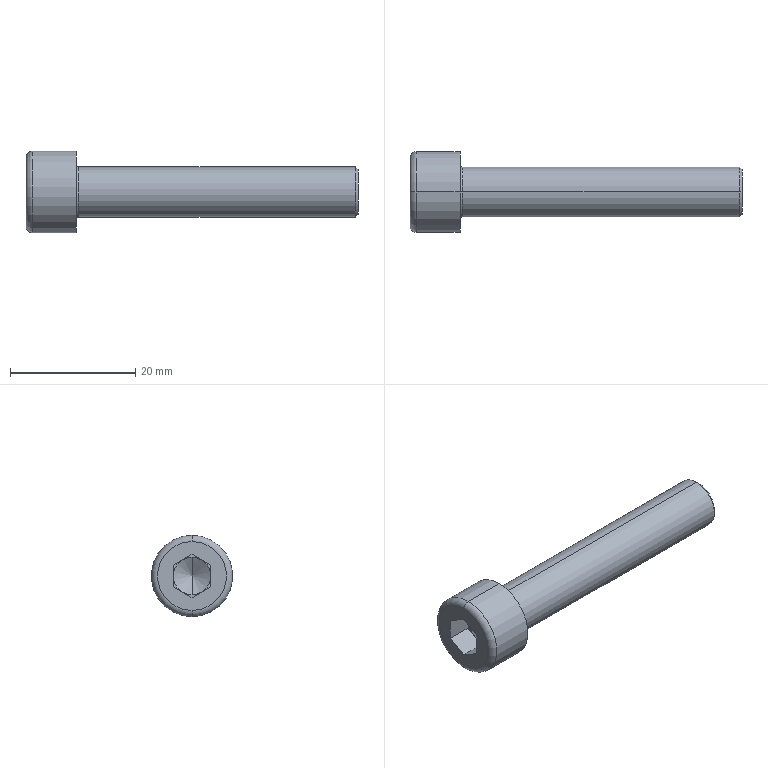Part | NX | features BREP 1 | 1 solid | 27 faces | box 53 x 13 x 13 mm | volume 3173 mm3 | plane 15 | torus 4 | cylinder 4 | cone 4 | commonest cylinder face diameters 8 x2 13 x2
STEP:
#1=CARTESIAN_POINT('',(8.4,0.,4.));
#2=VERTEX_POINT('',#1);
#3=CARTESIAN_POINT('',(8.,0.,4.4));
#4=VERTEX_POINT('',#3);
#5=CARTESIAN_POINT('',(8.4,0.,4.4));
#6=DIRECTION('',(0.,1.,0.));
#7=DIRECTION('',(0.,0.,1.));
#8=AXIS2_PLACEMENT_3D('',#5,#6,#7);
#9=CIRCLE('',#8,0.4);
#10=EDGE_CURVE('',#2,#4,#9,.T.);
#11=ORIENTED_EDGE('',*,*,#10,.F.);
#12=CARTESIAN_POINT('',(8.4,0.,-4.));
#13=VERTEX_POINT('',#12);
#14=CARTESIAN_POINT('',(8.4,0.,0.));
#15=DIRECTION('',(1.,0.,0.));
#16=DIRECTION('',(0.,0.,-1.));
#17=AXIS2_PLACEMENT_3D('',#14,#15,#16);
#18=CIRCLE('',#17,4.);
#19=EDGE_CURVE('',#13,#2,#18,.T.);
#20=ORIENTED_EDGE('',*,*,#19,.F.);
#21=CARTESIAN_POINT('',(8.,0.,-4.4));
#22=VERTEX_POINT('',#21);
#23=CARTESIAN_POINT('',(8.4,0.,-4.4));
#24=DIRECTION('',(0.,-1.,0.));
#25=DIRECTION('',(0.,0.,-1.));
#26=AXIS2_PLACEMENT_3D('',#23,#24,#25);
#27=CIRCLE('',#26,0.4);
#28=EDGE_CURVE('',#13,#22,#27,.T.);
#29=ORIENTED_EDGE('',*,*,#28,.T.);
#30=CARTESIAN_POINT('',(8.,0.,0.));
#31=DIRECTION('',(-1.,0.,0.));
#32=DIRECTION('',(0.,0.,-1.));
#33=AXIS2_PLACEMENT_3D('',#30,#31,#32);
#34=CIRCLE('',#33,4.4);
#35=EDGE_CURVE('',#4,#22,#34,.T.);
#36=ORIENTED_EDGE('',*,*,#35,.F.);
#37=EDGE_LOOP('',(#11,#20,#29,#36));
#38=FACE_BOUND('',#37,.T.);
#39=CARTESIAN_POINT('',(8.4,0.,0.));
#40=DIRECTION('',(1.,0.,0.));
#41=DIRECTION('',(0.,0.,1.));
#42=AXIS2_PLACEMENT_3D('',#39,#40,#41);
#43=TOROIDAL_SURFACE('',#42,4.4,0.4);
#44=ADVANCED_FACE('',(#38),#43,.F.);
#45=CARTESIAN_POINT('',(52.6,0.,4.));
#46=VERTEX_POINT('',#45);
#47=CARTESIAN_POINT('',(52.6,0.,-4.));
#48=VERTEX_POINT('',#47);
#49=CARTESIAN_POINT('',(52.6,0.,0.));
#50=DIRECTION('',(-1.,0.,0.));
#51=DIRECTION('',(0.,0.,-1.));
#52=AXIS2_PLACEMENT_3D('',#49,#50,#51);
#53=CIRCLE('',#52,4.);
#54=EDGE_CURVE('',#46,#48,#53,.T.);
#55=ORIENTED_EDGE('',*,*,#54,.T.);
#56=CARTESIAN_POINT('',(53.,0.,-4.));
#57=DIRECTION('',(-1.,0.,0.));
#58=VECTOR('',#57,1000.);
#59=LINE('',#56,#58);
#60=EDGE_CURVE('',#48,#13,#59,.T.);
#61=ORIENTED_EDGE('',*,*,#60,.T.);
#62=ORIENTED_EDGE('',*,*,#19,.T.);
#63=CARTESIAN_POINT('',(53.,0.,4.));
#64=DIRECTION('',(-1.,0.,0.));
#65=VECTOR('',#64,1000.);
#66=LINE('',#63,#65);
#67=EDGE_CURVE('',#46,#2,#66,.T.);
#68=ORIENTED_EDGE('',*,*,#67,.F.);
#69=EDGE_LOOP('',(#55,#61,#62,#68));
#70=FACE_BOUND('',#69,.T.);
#71=CARTESIAN_POINT('',(53.,0.,0.));
#72=DIRECTION('',(-1.,0.,0.));
#73=DIRECTION('',(0.,0.,-1.));
#74=AXIS2_PLACEMENT_3D('',#71,#72,#73);
#75=CYLINDRICAL_SURFACE('',#74,4.);
#76=ADVANCED_FACE('',(#70),#75,.T.);
#77=CARTESIAN_POINT('',(8.4,0.,0.));
#78=DIRECTION('',(1.,0.,0.));
#79=DIRECTION('',(0.,0.,-1.));
#80=AXIS2_PLACEMENT_3D('',#77,#78,#79);
#81=CIRCLE('',#80,4.);
#82=EDGE_CURVE('',#2,#13,#81,.T.);
#83=ORIENTED_EDGE('',*,*,#82,.F.);
#84=ORIENTED_EDGE('',*,*,#10,.T.);
#85=CARTESIAN_POINT('',(8.,0.,0.));
#86=DIRECTION('',(-1.,0.,0.));
#87=DIRECTION('',(0.,0.,-1.));
#88=AXIS2_PLACEMENT_3D('',#85,#86,#87);
#89=CIRCLE('',#88,4.4);
#90=EDGE_CURVE('',#22,#4,#89,.T.);
#91=ORIENTED_EDGE('',*,*,#90,.F.);
#92=ORIENTED_EDGE('',*,*,#28,.F.);
#93=EDGE_LOOP('',(#83,#84,#91,#92));
#94=FACE_BOUND('',#93,.T.);
#95=CARTESIAN_POINT('',(8.4,0.,0.));
#96=DIRECTION('',(1.,0.,0.));
#97=DIRECTION('',(0.,0.,1.));
#98=AXIS2_PLACEMENT_3D('',#95,#96,#97);
#99=TOROIDAL_SURFACE('',#98,4.4,0.4);
#100=ADVANCED_FACE('',(#94),#99,.F.);
#101=ORIENTED_EDGE('',*,*,#90,.T.);
#102=ORIENTED_EDGE('',*,*,#35,.T.);
#103=EDGE_LOOP('',(#101,#102));
#104=FACE_BOUND('',#103,.T.);
#105=CARTESIAN_POINT('',(8.,0.,6.5));
#106=VERTEX_POINT('',#105);
#107=CARTESIAN_POINT('',(8.,0.,-6.5));
#108=VERTEX_POINT('',#107);
#109=CARTESIAN_POINT('',(8.,0.,0.));
#110=DIRECTION('',(1.,0.,0.));
#111=DIRECTION('',(0.,0.,-1.));
#112=AXIS2_PLACEMENT_3D('',#109,#110,#111);
#113=CIRCLE('',#112,6.5);
#114=EDGE_CURVE('',#106,#108,#113,.T.);
#115=ORIENTED_EDGE('',*,*,#114,.T.);
#116=CARTESIAN_POINT('',(8.,0.,0.));
#117=DIRECTION('',(1.,0.,0.));
#118=DIRECTION('',(0.,0.,-1.));
#119=AXIS2_PLACEMENT_3D('',#116,#117,#118);
#120=CIRCLE('',#119,6.5);
#121=EDGE_CURVE('',#108,#106,#120,.T.);
#122=ORIENTED_EDGE('',*,*,#121,.T.);
#123=EDGE_LOOP('',(#115,#122));
#124=FACE_BOUND('',#123,.T.);
#125=CARTESIAN_POINT('',(8.,0.,0.));
#126=DIRECTION('',(1.,0.,0.));
#127=DIRECTION('',(0.,0.,1.));
#128=AXIS2_PLACEMENT_3D('',#125,#126,#127);
#129=PLANE('',#128);
#130=ADVANCED_FACE('',(#104,#124),#129,.T.);
#131=ORIENTED_EDGE('',*,*,#60,.F.);
#132=CARTESIAN_POINT('',(52.6,0.,0.));
#133=DIRECTION('',(-1.,0.,0.));
#134=DIRECTION('',(0.,0.,-1.));
#135=AXIS2_PLACEMENT_3D('',#132,#133,#134);
#136=CIRCLE('',#135,4.);
#137=EDGE_CURVE('',#48,#46,#136,.T.);
#138=ORIENTED_EDGE('',*,*,#137,.T.);
#139=ORIENTED_EDGE('',*,*,#67,.T.);
#140=ORIENTED_EDGE('',*,*,#82,.T.);
#141=EDGE_LOOP('',(#131,#138,#139,#140));
#142=FACE_BOUND('',#141,.T.);
#143=CARTESIAN_POINT('',(53.,0.,0.));
#144=DIRECTION('',(-1.,0.,0.));
#145=DIRECTION('',(0.,0.,-1.));
#146=AXIS2_PLACEMENT_3D('',#143,#144,#145);
#147=CYLINDRICAL_SURFACE('',#146,4.);
#148=ADVANCED_FACE('',(#142),#147,.T.);
#149=CARTESIAN_POINT('',(53.,0.,-3.6));
#150=VERTEX_POINT('',#149);
#151=CARTESIAN_POINT('',(53.,0.,3.6));
#152=VERTEX_POINT('',#151);
#153=CARTESIAN_POINT('',(53.,0.,0.));
#154=DIRECTION('',(1.,0.,0.));
#155=DIRECTION('',(0.,0.,-1.));
#156=AXIS2_PLACEMENT_3D('',#153,#154,#155);
#157=CIRCLE('',#156,3.6);
#158=EDGE_CURVE('',#150,#152,#157,.T.);
#159=ORIENTED_EDGE('',*,*,#158,.F.);
#160=CARTESIAN_POINT('',(53.,0.,-3.6));
#161=DIRECTION('',(-0.7071,0.,-0.7071));
#162=VECTOR('',#161,1000.);
#163=LINE('',#160,#162);
#164=EDGE_CURVE('',#150,#48,#163,.T.);
#165=ORIENTED_EDGE('',*,*,#164,.T.);
#166=ORIENTED_EDGE('',*,*,#54,.F.);
#167=CARTESIAN_POINT('',(53.,0.,3.6));
#168=DIRECTION('',(-0.7071,0.,0.7071));
#169=VECTOR('',#168,1000.);
#170=LINE('',#167,#169);
#171=EDGE_CURVE('',#152,#46,#170,.T.);
#172=ORIENTED_EDGE('',*,*,#171,.F.);
#173=EDGE_LOOP('',(#159,#165,#166,#172));
#174=FACE_BOUND('',#173,.T.);
#175=CARTESIAN_POINT('',(53.,0.,0.));
#176=DIRECTION('',(-1.,0.,0.));
#177=DIRECTION('',(0.,0.,-1.));
#178=AXIS2_PLACEMENT_3D('',#175,#176,#177);
#179=CONICAL_SURFACE('',#178,3.6,0.7854);
#180=ADVANCED_FACE('',(#174),#179,.T.);
#181=CARTESIAN_POINT('',(1.,0.,-6.5));
#182=VERTEX_POINT('',#181);
#183=CARTESIAN_POINT('',(8.,0.,-6.5));
#184=DIRECTION('',(-1.,0.,0.));
#185=VECTOR('',#184,1000.);
#186=LINE('',#183,#185);
#187=EDGE_CURVE('',#182,#108,#186,.F.);
#188=ORIENTED_EDGE('',*,*,#187,.T.);
#189=ORIENTED_EDGE('',*,*,#114,.F.);
#190=CARTESIAN_POINT('',(1.,0.,6.5));
#191=VERTEX_POINT('',#190);
#192=CARTESIAN_POINT('',(8.,0.,6.5));
#193=DIRECTION('',(-1.,0.,0.));
#194=VECTOR('',#193,1000.);
#195=LINE('',#192,#194);
#196=EDGE_CURVE('',#191,#106,#195,.F.);
#197=ORIENTED_EDGE('',*,*,#196,.F.);
#198=CARTESIAN_POINT('',(1.,0.,0.));
#199=DIRECTION('',(1.,0.,0.));
#200=DIRECTION('',(0.,0.,-1.));
#201=AXIS2_PLACEMENT_3D('',#198,#199,#200);
#202=CIRCLE('',#201,6.5);
#203=EDGE_CURVE('',#191,#182,#202,.T.);
#204=ORIENTED_EDGE('',*,*,#203,.T.);
#205=EDGE_LOOP('',(#188,#189,#197,#204));
#206=FACE_BOUND('',#205,.T.);
#207=CARTESIAN_POINT('',(8.,0.,0.));
#208=DIRECTION('',(-1.,0.,0.));
#209=DIRECTION('',(0.,0.,-1.));
#210=AXIS2_PLACEMENT_3D('',#207,#208,#209);
#211=CYLINDRICAL_SURFACE('',#210,6.5);
#212=ADVANCED_FACE('',(#206),#211,.T.);
#213=ORIENTED_EDGE('',*,*,#121,.F.);
#214=ORIENTED_EDGE('',*,*,#187,.F.);
#215=CARTESIAN_POINT('',(1.,0.,0.));
#216=DIRECTION('',(1.,0.,0.));
#217=DIRECTION('',(0.,0.,-1.));
#218=AXIS2_PLACEMENT_3D('',#215,#216,#217);
#219=CIRCLE('',#218,6.5);
#220=EDGE_CURVE('',#182,#191,#219,.T.);
#221=ORIENTED_EDGE('',*,*,#220,.T.);
#222=ORIENTED_EDGE('',*,*,#196,.T.);
#223=EDGE_LOOP('',(#213,#214,#221,#222));
#224=FACE_BOUND('',#223,.T.);
#225=CARTESIAN_POINT('',(8.,0.,0.));
#226=DIRECTION('',(-1.,0.,0.));
#227=DIRECTION('',(0.,0.,-1.));
#228=AXIS2_PLACEMENT_3D('',#225,#226,#227);
#229=CYLINDRICAL_SURFACE('',#228,6.5);
#230=ADVANCED_FACE('',(#224),#229,.T.);
#231=ORIENTED_EDGE('',*,*,#164,.F.);
#232=CARTESIAN_POINT('',(53.,0.,0.));
#233=DIRECTION('',(1.,0.,0.));
#234=DIRECTION('',(0.,0.,-1.));
#235=AXIS2_PLACEMENT_3D('',#232,#233,#234);
#236=CIRCLE('',#235,3.6);
#237=EDGE_CURVE('',#152,#150,#236,.T.);
#238=ORIENTED_EDGE('',*,*,#237,.F.);
#239=ORIENTED_EDGE('',*,*,#171,.T.);
#240=ORIENTED_EDGE('',*,*,#137,.F.);
#241=EDGE_LOOP('',(#231,#238,#239,#240));
#242=FACE_BOUND('',#241,.T.);
#243=CARTESIAN_POINT('',(53.,0.,0.));
#244=DIRECTION('',(-1.,0.,0.));
#245=DIRECTION('',(0.,0.,-1.));
#246=AXIS2_PLACEMENT_3D('',#243,#244,#245);
#247=CONICAL_SURFACE('',#246,3.6,0.7854);
#248=ADVANCED_FACE('',(#242),#247,.T.);
#249=ORIENTED_EDGE('',*,*,#237,.T.);
#250=ORIENTED_EDGE('',*,*,#158,.T.);
#251=EDGE_LOOP('',(#249,#250));
#252=FACE_BOUND('',#251,.T.);
#253=CARTESIAN_POINT('',(53.,0.,0.));
#254=DIRECTION('',(1.,0.,0.));
#255=DIRECTION('',(0.,0.,1.));
#256=AXIS2_PLACEMENT_3D('',#253,#254,#255);
#257=PLANE('',#256);
#258=ADVANCED_FACE('',(#252),#257,.T.);
#259=CARTESIAN_POINT('',(0.,0.,5.5));
#260=VERTEX_POINT('',#259);
#261=CARTESIAN_POINT('',(1.,0.,5.5));
#262=DIRECTION('',(0.,1.,0.));
#263=DIRECTION('',(0.,0.,1.));
#264=AXIS2_PLACEMENT_3D('',#261,#262,#263);
#265=CIRCLE('',#264,1.);
#266=EDGE_CURVE('',#260,#191,#265,.T.);
#267=ORIENTED_EDGE('',*,*,#266,.F.);
#268=CARTESIAN_POINT('',(0.,0.,-5.5));
#269=VERTEX_POINT('',#268);
#270=CARTESIAN_POINT('',(0.,0.,0.));
#271=DIRECTION('',(-1.,0.,0.));
#272=DIRECTION('',(0.,0.,-1.));
#273=AXIS2_PLACEMENT_3D('',#270,#271,#272);
#274=CIRCLE('',#273,5.5);
#275=EDGE_CURVE('',#269,#260,#274,.T.);
#276=ORIENTED_EDGE('',*,*,#275,.F.);
#277=CARTESIAN_POINT('',(1.,0.,-5.5));
#278=DIRECTION('',(0.,-1.,0.));
#279=DIRECTION('',(0.,0.,-1.));
#280=AXIS2_PLACEMENT_3D('',#277,#278,#279);
#281=CIRCLE('',#280,1.);
#282=EDGE_CURVE('',#269,#182,#281,.T.);
#283=ORIENTED_EDGE('',*,*,#282,.T.);
#284=ORIENTED_EDGE('',*,*,#203,.F.);
#285=EDGE_LOOP('',(#267,#276,#283,#284));
#286=FACE_BOUND('',#285,.T.);
#287=CARTESIAN_POINT('',(1.,0.,0.));
#288=DIRECTION('',(1.,0.,0.));
#289=DIRECTION('',(0.,0.,1.));
#290=AXIS2_PLACEMENT_3D('',#287,#288,#289);
#291=TOROIDAL_SURFACE('',#290,5.5,1.);
#292=ADVANCED_FACE('',(#286),#291,.T.);
#293=CARTESIAN_POINT('',(0.,0.,0.));
#294=DIRECTION('',(-1.,0.,0.));
#295=DIRECTION('',(0.,0.,-1.));
#296=AXIS2_PLACEMENT_3D('',#293,#294,#295);
#297=CIRCLE('',#296,5.5);
#298=EDGE_CURVE('',#260,#269,#297,.T.);
#299=ORIENTED_EDGE('',*,*,#298,.F.);
#300=ORIENTED_EDGE('',*,*,#266,.T.);
#301=ORIENTED_EDGE('',*,*,#220,.F.);
#302=ORIENTED_EDGE('',*,*,#282,.F.);
#303=EDGE_LOOP('',(#299,#300,#301,#302));
#304=FACE_BOUND('',#303,.T.);
#305=CARTESIAN_POINT('',(1.,0.,0.));
#306=DIRECTION('',(1.,0.,0.));
#307=DIRECTION('',(0.,0.,1.));
#308=AXIS2_PLACEMENT_3D('',#305,#306,#307);
#309=TOROIDAL_SURFACE('',#308,5.5,1.);
#310=ADVANCED_FACE('',(#304),#309,.T.);
#311=ORIENTED_EDGE('',*,*,#275,.T.);
#312=ORIENTED_EDGE('',*,*,#298,.T.);
#313=EDGE_LOOP('',(#311,#312));
#314=FACE_BOUND('',#313,.T.);
#315=CARTESIAN_POINT('',(0.,-3.,-1.732));
#316=VERTEX_POINT('',#315);
#317=CARTESIAN_POINT('',(0.,0.,-3.464));
#318=VERTEX_POINT('',#317);
#319=CARTESIAN_POINT('',(0.,-3.,-1.732));
#320=DIRECTION('',(0.,0.866,-0.5));
#321=VECTOR('',#320,1000.);
#322=LINE('',#319,#321);
#323=EDGE_CURVE('',#316,#318,#322,.T.);
#324=ORIENTED_EDGE('',*,*,#323,.T.);
#325=CARTESIAN_POINT('',(0.,3.,-1.732));
#326=VERTEX_POINT('',#325);
#327=CARTESIAN_POINT('',(0.,0.,-3.464));
#328=DIRECTION('',(0.,0.866,0.5));
#329=VECTOR('',#328,1000.);
#330=LINE('',#327,#329);
#331=EDGE_CURVE('',#318,#326,#330,.T.);
#332=ORIENTED_EDGE('',*,*,#331,.T.);
#333=CARTESIAN_POINT('',(0.,3.,1.732));
#334=VERTEX_POINT('',#333);
#335=CARTESIAN_POINT('',(0.,3.,-1.732));
#336=DIRECTION('',(0.,0.,1.));
#337=VECTOR('',#336,1000.);
#338=LINE('',#335,#337);
#339=EDGE_CURVE('',#326,#334,#338,.T.);
#340=ORIENTED_EDGE('',*,*,#339,.T.);
#341=CARTESIAN_POINT('',(0.,0.,3.464));
#342=VERTEX_POINT('',#341);
#343=CARTESIAN_POINT('',(0.,3.,1.732));
#344=DIRECTION('',(0.,-0.866,0.5));
#345=VECTOR('',#344,1000.);
#346=LINE('',#343,#345);
#347=EDGE_CURVE('',#334,#342,#346,.T.);
#348=ORIENTED_EDGE('',*,*,#347,.T.);
#349=CARTESIAN_POINT('',(0.,-3.,1.732));
#350=VERTEX_POINT('',#349);
#351=CARTESIAN_POINT('',(0.,0.,3.464));
#352=DIRECTION('',(0.,-0.866,-0.5));
#353=VECTOR('',#352,1000.);
#354=LINE('',#351,#353);
#355=EDGE_CURVE('',#342,#350,#354,.T.);
#356=ORIENTED_EDGE('',*,*,#355,.T.);
#357=CARTESIAN_POINT('',(0.,-3.,1.732));
#358=DIRECTION('',(0.,0.,-1.));
#359=VECTOR('',#358,1000.);
#360=LINE('',#357,#359);
#361=EDGE_CURVE('',#350,#316,#360,.T.);
#362=ORIENTED_EDGE('',*,*,#361,.T.);
#363=EDGE_LOOP('',(#324,#332,#340,#348,#356,#362));
#364=FACE_BOUND('',#363,.T.);
#365=CARTESIAN_POINT('',(0.,0.,0.));
#366=DIRECTION('',(1.,0.,0.));
#367=DIRECTION('',(0.,0.,1.));
#368=AXIS2_PLACEMENT_3D('',#365,#366,#367);
#369=PLANE('',#368);
#370=ADVANCED_FACE('',(#314,#364),#369,.F.);
#371=ORIENTED_EDGE('',*,*,#361,.F.);
#372=CARTESIAN_POINT('',(4.,-3.,1.732));
#373=VERTEX_POINT('',#372);
#374=CARTESIAN_POINT('',(4.,-3.,1.732));
#375=DIRECTION('',(-1.,0.,0.));
#376=VECTOR('',#375,1000.);
#377=LINE('',#374,#376);
#378=EDGE_CURVE('',#373,#350,#377,.T.);
#379=ORIENTED_EDGE('',*,*,#378,.F.);
#380=CARTESIAN_POINT('',(4.,-3.,0.));
#381=VERTEX_POINT('',#380);
#382=CARTESIAN_POINT('',(4.,-3.,1.732));
#383=DIRECTION('',(0.,0.,-1.));
#384=VECTOR('',#383,1000.);
#385=LINE('',#382,#384);
#386=EDGE_CURVE('',#373,#381,#385,.T.);
#387=ORIENTED_EDGE('',*,*,#386,.T.);
#388=CARTESIAN_POINT('',(4.,-3.,-1.732));
#389=VERTEX_POINT('',#388);
#390=CARTESIAN_POINT('',(4.,-3.,1.732));
#391=DIRECTION('',(0.,0.,-1.));
#392=VECTOR('',#391,1000.);
#393=LINE('',#390,#392);
#394=EDGE_CURVE('',#381,#389,#393,.T.);
#395=ORIENTED_EDGE('',*,*,#394,.T.);
#396=CARTESIAN_POINT('',(4.,-3.,-1.732));
#397=DIRECTION('',(-1.,0.,0.));
#398=VECTOR('',#397,1000.);
#399=LINE('',#396,#398);
#400=EDGE_CURVE('',#389,#316,#399,.T.);
#401=ORIENTED_EDGE('',*,*,#400,.T.);
#402=EDGE_LOOP('',(#371,#379,#387,#395,#401));
#403=FACE_BOUND('',#402,.T.);
#404=CARTESIAN_POINT('',(4.,-3.,1.732));
#405=DIRECTION('',(0.,1.,0.));
#406=DIRECTION('',(0.,0.,-1.));
#407=AXIS2_PLACEMENT_3D('',#404,#405,#406);
#408=PLANE('',#407);
#409=ADVANCED_FACE('',(#403),#408,.T.);
#410=ORIENTED_EDGE('',*,*,#347,.F.);
#411=CARTESIAN_POINT('',(4.,3.,1.732));
#412=VERTEX_POINT('',#411);
#413=CARTESIAN_POINT('',(4.,3.,1.732));
#414=DIRECTION('',(-1.,0.,0.));
#415=VECTOR('',#414,1000.);
#416=LINE('',#413,#415);
#417=EDGE_CURVE('',#412,#334,#416,.T.);
#418=ORIENTED_EDGE('',*,*,#417,.F.);
#419=CARTESIAN_POINT('',(4.,1.5,2.598));
#420=VERTEX_POINT('',#419);
#421=CARTESIAN_POINT('',(4.,3.,1.732));
#422=DIRECTION('',(0.,-0.866,0.5));
#423=VECTOR('',#422,1000.);
#424=LINE('',#421,#423);
#425=EDGE_CURVE('',#412,#420,#424,.T.);
#426=ORIENTED_EDGE('',*,*,#425,.T.);
#427=CARTESIAN_POINT('',(4.,0.,3.464));
#428=VERTEX_POINT('',#427);
#429=CARTESIAN_POINT('',(4.,3.,1.732));
#430=DIRECTION('',(0.,-0.866,0.5));
#431=VECTOR('',#430,1000.);
#432=LINE('',#429,#431);
#433=EDGE_CURVE('',#420,#428,#432,.T.);
#434=ORIENTED_EDGE('',*,*,#433,.T.);
#435=CARTESIAN_POINT('',(4.,0.,3.464));
#436=DIRECTION('',(-1.,0.,0.));
#437=VECTOR('',#436,1000.);
#438=LINE('',#435,#437);
#439=EDGE_CURVE('',#428,#342,#438,.T.);
#440=ORIENTED_EDGE('',*,*,#439,.T.);
#441=EDGE_LOOP('',(#410,#418,#426,#434,#440));
#442=FACE_BOUND('',#441,.T.);
#443=CARTESIAN_POINT('',(4.,3.,1.732));
#444=DIRECTION('',(0.,-0.5,-0.866));
#445=DIRECTION('',(0.,-0.866,0.5));
#446=AXIS2_PLACEMENT_3D('',#443,#444,#445);
#447=PLANE('',#446);
#448=ADVANCED_FACE('',(#442),#447,.T.);
#449=ORIENTED_EDGE('',*,*,#331,.F.);
#450=CARTESIAN_POINT('',(4.,0.,-3.464));
#451=VERTEX_POINT('',#450);
#452=CARTESIAN_POINT('',(4.,0.,-3.464));
#453=DIRECTION('',(-1.,0.,0.));
#454=VECTOR('',#453,1000.);
#455=LINE('',#452,#454);
#456=EDGE_CURVE('',#451,#318,#455,.T.);
#457=ORIENTED_EDGE('',*,*,#456,.F.);
#458=CARTESIAN_POINT('',(4.,1.5,-2.598));
#459=VERTEX_POINT('',#458);
#460=CARTESIAN_POINT('',(4.,0.,-3.464));
#461=DIRECTION('',(0.,0.866,0.5));
#462=VECTOR('',#461,1000.);
#463=LINE('',#460,#462);
#464=EDGE_CURVE('',#451,#459,#463,.T.);
#465=ORIENTED_EDGE('',*,*,#464,.T.);
#466=CARTESIAN_POINT('',(4.,3.,-1.732));
#467=VERTEX_POINT('',#466);
#468=CARTESIAN_POINT('',(4.,0.,-3.464));
#469=DIRECTION('',(0.,0.866,0.5));
#470=VECTOR('',#469,1000.);
#471=LINE('',#468,#470);
#472=EDGE_CURVE('',#459,#467,#471,.T.);
#473=ORIENTED_EDGE('',*,*,#472,.T.);
#474=CARTESIAN_POINT('',(4.,3.,-1.732));
#475=DIRECTION('',(-1.,0.,0.));
#476=VECTOR('',#475,1000.);
#477=LINE('',#474,#476);
#478=EDGE_CURVE('',#467,#326,#477,.T.);
#479=ORIENTED_EDGE('',*,*,#478,.T.);
#480=EDGE_LOOP('',(#449,#457,#465,#473,#479));
#481=FACE_BOUND('',#480,.T.);
#482=CARTESIAN_POINT('',(4.,0.,-3.464));
#483=DIRECTION('',(0.,-0.5,0.866));
#484=DIRECTION('',(0.,0.866,0.5));
#485=AXIS2_PLACEMENT_3D('',#482,#483,#484);
#486=PLANE('',#485);
#487=ADVANCED_FACE('',(#481),#486,.T.);
#488=ORIENTED_EDGE('',*,*,#323,.F.);
#489=ORIENTED_EDGE('',*,*,#400,.F.);
#490=CARTESIAN_POINT('',(4.,-1.5,-2.598));
#491=VERTEX_POINT('',#490);
#492=CARTESIAN_POINT('',(4.,-3.,-1.732));
#493=DIRECTION('',(0.,0.866,-0.5));
#494=VECTOR('',#493,1000.);
#495=LINE('',#492,#494);
#496=EDGE_CURVE('',#389,#491,#495,.T.);
#497=ORIENTED_EDGE('',*,*,#496,.T.);
#498=CARTESIAN_POINT('',(4.,-3.,-1.732));
#499=DIRECTION('',(0.,0.866,-0.5));
#500=VECTOR('',#499,1000.);
#501=LINE('',#498,#500);
#502=EDGE_CURVE('',#491,#451,#501,.T.);
#503=ORIENTED_EDGE('',*,*,#502,.T.);
#504=ORIENTED_EDGE('',*,*,#456,.T.);
#505=EDGE_LOOP('',(#488,#489,#497,#503,#504));
#506=FACE_BOUND('',#505,.T.);
#507=CARTESIAN_POINT('',(4.,-3.,-1.732));
#508=DIRECTION('',(0.,0.5,0.866));
#509=DIRECTION('',(0.,0.866,-0.5));
#510=AXIS2_PLACEMENT_3D('',#507,#508,#509);
#511=PLANE('',#510);
#512=ADVANCED_FACE('',(#506),#511,.T.);
#513=ORIENTED_EDGE('',*,*,#339,.F.);
#514=ORIENTED_EDGE('',*,*,#478,.F.);
#515=CARTESIAN_POINT('',(4.,3.,0.));
#516=VERTEX_POINT('',#515);
#517=CARTESIAN_POINT('',(4.,3.,-1.732));
#518=DIRECTION('',(0.,0.,1.));
#519=VECTOR('',#518,1000.);
#520=LINE('',#517,#519);
#521=EDGE_CURVE('',#467,#516,#520,.T.);
#522=ORIENTED_EDGE('',*,*,#521,.T.);
#523=CARTESIAN_POINT('',(4.,3.,-1.732));
#524=DIRECTION('',(0.,0.,1.));
#525=VECTOR('',#524,1000.);
#526=LINE('',#523,#525);
#527=EDGE_CURVE('',#516,#412,#526,.T.);
#528=ORIENTED_EDGE('',*,*,#527,.T.);
#529=ORIENTED_EDGE('',*,*,#417,.T.);
#530=EDGE_LOOP('',(#513,#514,#522,#528,#529));
#531=FACE_BOUND('',#530,.T.);
#532=CARTESIAN_POINT('',(4.,3.,-1.732));
#533=DIRECTION('',(0.,-1.,0.));
#534=DIRECTION('',(0.,0.,1.));
#535=AXIS2_PLACEMENT_3D('',#532,#533,#534);
#536=PLANE('',#535);
#537=ADVANCED_FACE('',(#531),#536,.T.);
#538=ORIENTED_EDGE('',*,*,#355,.F.);
#539=ORIENTED_EDGE('',*,*,#439,.F.);
#540=CARTESIAN_POINT('',(4.,-1.5,2.598));
#541=VERTEX_POINT('',#540);
#542=CARTESIAN_POINT('',(4.,0.,3.464));
#543=DIRECTION('',(0.,-0.866,-0.5));
#544=VECTOR('',#543,1000.);
#545=LINE('',#542,#544);
#546=EDGE_CURVE('',#428,#541,#545,.T.);
#547=ORIENTED_EDGE('',*,*,#546,.T.);
#548=CARTESIAN_POINT('',(4.,0.,3.464));
#549=DIRECTION('',(0.,-0.866,-0.5));
#550=VECTOR('',#549,1000.);
#551=LINE('',#548,#550);
#552=EDGE_CURVE('',#541,#373,#551,.T.);
#553=ORIENTED_EDGE('',*,*,#552,.T.);
#554=ORIENTED_EDGE('',*,*,#378,.T.);
#555=EDGE_LOOP('',(#538,#539,#547,#553,#554));
#556=FACE_BOUND('',#555,.T.);
#557=CARTESIAN_POINT('',(4.,0.,3.464));
#558=DIRECTION('',(0.,0.5,-0.866));
#559=DIRECTION('',(0.,-0.866,-0.5));
#560=AXIS2_PLACEMENT_3D('',#557,#558,#559);
#561=PLANE('',#560);
#562=ADVANCED_FACE('',(#556),#561,.T.);
#563=ORIENTED_EDGE('',*,*,#552,.F.);
#564=CARTESIAN_POINT('',(4.,0.,0.));
#565=DIRECTION('',(1.,0.,0.));
#566=DIRECTION('',(0.,0.,-1.));
#567=AXIS2_PLACEMENT_3D('',#564,#565,#566);
#568=CIRCLE('',#567,3.);
#569=EDGE_CURVE('',#541,#381,#568,.T.);
#570=ORIENTED_EDGE('',*,*,#569,.T.);
#571=ORIENTED_EDGE('',*,*,#386,.F.);
#572=EDGE_LOOP('',(#563,#570,#571));
#573=FACE_BOUND('',#572,.T.);
#574=CARTESIAN_POINT('',(4.,0.,-3.464));
#575=DIRECTION('',(1.,0.,0.));
#576=DIRECTION('',(0.,0.,1.));
#577=AXIS2_PLACEMENT_3D('',#574,#575,#576);
#578=PLANE('',#577);
#579=ADVANCED_FACE('',(#573),#578,.F.);
#580=ORIENTED_EDGE('',*,*,#394,.F.);
#581=CARTESIAN_POINT('',(4.,0.,0.));
#582=DIRECTION('',(1.,0.,0.));
#583=DIRECTION('',(0.,0.,-1.));
#584=AXIS2_PLACEMENT_3D('',#581,#582,#583);
#585=CIRCLE('',#584,3.);
#586=EDGE_CURVE('',#381,#491,#585,.T.);
#587=ORIENTED_EDGE('',*,*,#586,.T.);
#588=ORIENTED_EDGE('',*,*,#496,.F.);
#589=EDGE_LOOP('',(#580,#587,#588));
#590=FACE_BOUND('',#589,.T.);
#591=CARTESIAN_POINT('',(4.,0.,-3.464));
#592=DIRECTION('',(1.,0.,0.));
#593=DIRECTION('',(0.,0.,1.));
#594=AXIS2_PLACEMENT_3D('',#591,#592,#593);
#595=PLANE('',#594);
#596=ADVANCED_FACE('',(#590),#595,.F.);
#597=ORIENTED_EDGE('',*,*,#527,.F.);
#598=CARTESIAN_POINT('',(4.,0.,0.));
#599=DIRECTION('',(1.,0.,0.));
#600=DIRECTION('',(0.,0.,-1.));
#601=AXIS2_PLACEMENT_3D('',#598,#599,#600);
#602=CIRCLE('',#601,3.);
#603=EDGE_CURVE('',#516,#420,#602,.T.);
#604=ORIENTED_EDGE('',*,*,#603,.T.);
#605=ORIENTED_EDGE('',*,*,#425,.F.);
#606=EDGE_LOOP('',(#597,#604,#605));
#607=FACE_BOUND('',#606,.T.);
#608=CARTESIAN_POINT('',(4.,0.,-3.464));
#609=DIRECTION('',(1.,0.,0.));
#610=DIRECTION('',(0.,0.,1.));
#611=AXIS2_PLACEMENT_3D('',#608,#609,#610);
#612=PLANE('',#611);
#613=ADVANCED_FACE('',(#607),#612,.F.);
#614=ORIENTED_EDGE('',*,*,#433,.F.);
#615=CARTESIAN_POINT('',(4.,0.,3.));
#616=VERTEX_POINT('',#615);
#617=CARTESIAN_POINT('',(4.,0.,0.));
#618=DIRECTION('',(1.,0.,0.));
#619=DIRECTION('',(0.,0.,-1.));
#620=AXIS2_PLACEMENT_3D('',#617,#618,#619);
#621=CIRCLE('',#620,3.);
#622=EDGE_CURVE('',#420,#616,#621,.T.);
#623=ORIENTED_EDGE('',*,*,#622,.T.);
#624=CARTESIAN_POINT('',(4.,0.,0.));
#625=DIRECTION('',(1.,0.,0.));
#626=DIRECTION('',(0.,0.,-1.));
#627=AXIS2_PLACEMENT_3D('',#624,#625,#626);
#628=CIRCLE('',#627,3.);
#629=EDGE_CURVE('',#616,#541,#628,.T.);
#630=ORIENTED_EDGE('',*,*,#629,.T.);
#631=ORIENTED_EDGE('',*,*,#546,.F.);
#632=EDGE_LOOP('',(#614,#623,#630,#631));
#633=FACE_BOUND('',#632,.T.);
#634=CARTESIAN_POINT('',(4.,0.,-3.464));
#635=DIRECTION('',(1.,0.,0.));
#636=DIRECTION('',(0.,0.,1.));
#637=AXIS2_PLACEMENT_3D('',#634,#635,#636);
#638=PLANE('',#637);
#639=ADVANCED_FACE('',(#633),#638,.F.);
#640=ORIENTED_EDGE('',*,*,#472,.F.);
#641=CARTESIAN_POINT('',(4.,0.,0.));
#642=DIRECTION('',(1.,0.,0.));
#643=DIRECTION('',(0.,0.,-1.));
#644=AXIS2_PLACEMENT_3D('',#641,#642,#643);
#645=CIRCLE('',#644,3.);
#646=EDGE_CURVE('',#459,#516,#645,.T.);
#647=ORIENTED_EDGE('',*,*,#646,.T.);
#648=ORIENTED_EDGE('',*,*,#521,.F.);
#649=EDGE_LOOP('',(#640,#647,#648));
#650=FACE_BOUND('',#649,.T.);
#651=CARTESIAN_POINT('',(4.,0.,-3.464));
#652=DIRECTION('',(1.,0.,0.));
#653=DIRECTION('',(0.,0.,1.));
#654=AXIS2_PLACEMENT_3D('',#651,#652,#653);
#655=PLANE('',#654);
#656=ADVANCED_FACE('',(#650),#655,.F.);
#657=ORIENTED_EDGE('',*,*,#502,.F.);
#658=CARTESIAN_POINT('',(4.,0.,-3.));
#659=VERTEX_POINT('',#658);
#660=CARTESIAN_POINT('',(4.,0.,0.));
#661=DIRECTION('',(1.,0.,0.));
#662=DIRECTION('',(0.,0.,-1.));
#663=AXIS2_PLACEMENT_3D('',#660,#661,#662);
#664=CIRCLE('',#663,3.);
#665=EDGE_CURVE('',#491,#659,#664,.T.);
#666=ORIENTED_EDGE('',*,*,#665,.T.);
#667=CARTESIAN_POINT('',(4.,0.,0.));
#668=DIRECTION('',(1.,0.,0.));
#669=DIRECTION('',(0.,0.,-1.));
#670=AXIS2_PLACEMENT_3D('',#667,#668,#669);
#671=CIRCLE('',#670,3.);
#672=EDGE_CURVE('',#659,#459,#671,.T.);
#673=ORIENTED_EDGE('',*,*,#672,.T.);
#674=ORIENTED_EDGE('',*,*,#464,.F.);
#675=EDGE_LOOP('',(#657,#666,#673,#674));
#676=FACE_BOUND('',#675,.T.);
#677=CARTESIAN_POINT('',(4.,0.,-3.464));
#678=DIRECTION('',(1.,0.,0.));
#679=DIRECTION('',(0.,0.,1.));
#680=AXIS2_PLACEMENT_3D('',#677,#678,#679);
#681=PLANE('',#680);
#682=ADVANCED_FACE('',(#676),#681,.F.);
#683=CARTESIAN_POINT('',(5.732,0.,0.));
#684=VERTEX_POINT('',#683);
#685=CARTESIAN_POINT('',(4.,0.,3.));
#686=DIRECTION('',(-0.5,0.,0.866));
#687=VECTOR('',#686,1000.);
#688=LINE('',#685,#687);
#689=EDGE_CURVE('',#684,#616,#688,.T.);
#690=ORIENTED_EDGE('',*,*,#689,.F.);
#691=CARTESIAN_POINT('',(4.,0.,-3.));
#692=DIRECTION('',(-0.5,0.,-0.866));
#693=VECTOR('',#692,1000.);
#694=LINE('',#691,#693);
#695=EDGE_CURVE('',#684,#659,#694,.T.);
#696=ORIENTED_EDGE('',*,*,#695,.T.);
#697=ORIENTED_EDGE('',*,*,#665,.F.);
#698=ORIENTED_EDGE('',*,*,#586,.F.);
#699=ORIENTED_EDGE('',*,*,#569,.F.);
#700=ORIENTED_EDGE('',*,*,#629,.F.);
#701=EDGE_LOOP('',(#690,#696,#697,#698,#699,#700));
#702=FACE_BOUND('',#701,.T.);
#703=CARTESIAN_POINT('',(4.,0.,0.));
#704=DIRECTION('',(-1.,0.,0.));
#705=DIRECTION('',(0.,0.,-1.));
#706=AXIS2_PLACEMENT_3D('',#703,#704,#705);
#707=CONICAL_SURFACE('',#706,3.,1.047);
#708=ADVANCED_FACE('',(#702),#707,.F.);
#709=ORIENTED_EDGE('',*,*,#695,.F.);
#710=ORIENTED_EDGE('',*,*,#689,.T.);
#711=ORIENTED_EDGE('',*,*,#622,.F.);
#712=ORIENTED_EDGE('',*,*,#603,.F.);
#713=ORIENTED_EDGE('',*,*,#646,.F.);
#714=ORIENTED_EDGE('',*,*,#672,.F.);
#715=EDGE_LOOP('',(#709,#710,#711,#712,#713,#714));
#716=FACE_BOUND('',#715,.T.);
#717=CARTESIAN_POINT('',(4.,0.,0.));
#718=DIRECTION('',(-1.,0.,0.));
#719=DIRECTION('',(0.,0.,-1.));
#720=AXIS2_PLACEMENT_3D('',#717,#718,#719);
#721=CONICAL_SURFACE('',#720,3.,1.047);
#722=ADVANCED_FACE('',(#716),#721,.F.);
#723=CLOSED_SHELL('',(#44,#76,#100,#130,#148,#180,#212,#230,#248,#258,#292,#310,#370,#409,#448,#487,#512,#537,#562,#579,#596,#613,#639,#656,#682,#708,#722));
#724=MANIFOLD_SOLID_BREP('',#723);
#725=(LENGTH_UNIT()NAMED_UNIT(*)SI_UNIT(.MILLI.,.METRE.));
#726=UNCERTAINTY_MEASURE_WITH_UNIT(LENGTH_MEASURE(0.00001),#725,'','');
#727=(NAMED_UNIT(*)PLANE_ANGLE_UNIT()SI_UNIT($,.RADIAN.));
#728=(NAMED_UNIT(*)SI_UNIT($,.STERADIAN.)SOLID_ANGLE_UNIT());
#729=(GEOMETRIC_REPRESENTATION_CONTEXT(3)GLOBAL_UNCERTAINTY_ASSIGNED_CONTEXT((#726))GLOBAL_UNIT_ASSIGNED_CONTEXT((#725,#727,#728))REPRESENTATION_CONTEXT('',''));
#730=ADVANCED_BREP_SHAPE_REPRESENTATION('',(#724),#729);